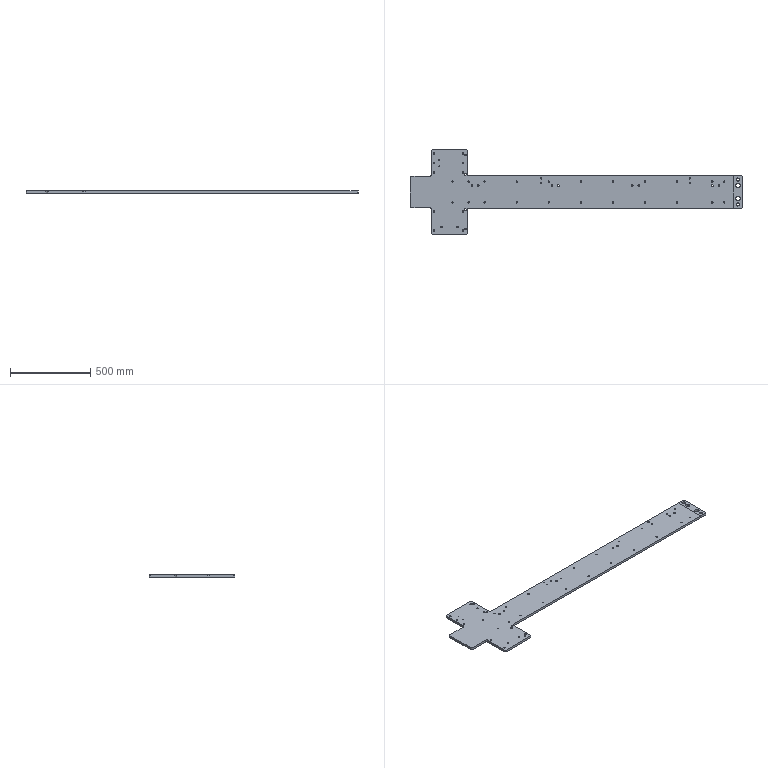Part | STEP file | J452-EBZ05-01-08-Part-1 | 1 solid | 170 faces | box 2070 x 530 x 15 mm | volume 7252228 mm3 | cylinder 124 | plane 30 | cone 16 | commonest cylinder face diameters 8 x60 10 x40 6.8 x8 20 x8 5 x4 27 x4